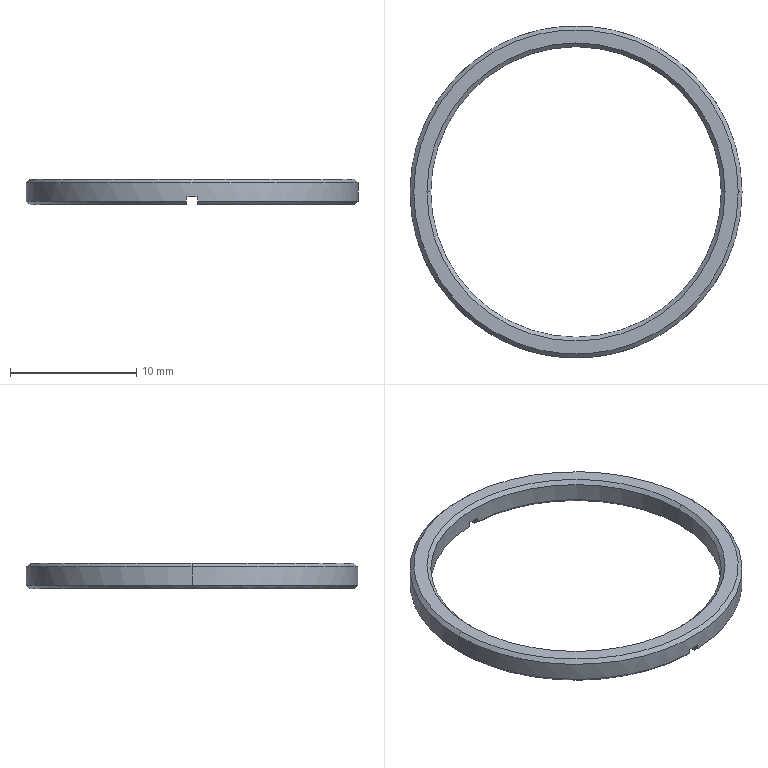Part | STEP file | 1 solid | 27 faces | box 26.29 x 26.29 x 2.05 mm | volume 245.399 mm3 | cone 10 | plane 9 | cylinder 8 | commonest cylinder face diameters 0.1 x4 23 x2 26.29 x2
STEP:
#1=CARTESIAN_POINT('',(12.845,0.,2.05));
#2=VERTEX_POINT('',#1);
#3=CARTESIAN_POINT('',(-12.845,0.,2.05));
#4=VERTEX_POINT('',#3);
#5=CARTESIAN_POINT('',(0.,0.,2.05));
#6=DIRECTION('',(0.,0.,1.));
#7=DIRECTION('',(1.,0.,0.));
#8=AXIS2_PLACEMENT_3D('',#5,#6,#7);
#9=CIRCLE('',#8,12.845);
#10=EDGE_CURVE('',#2,#4,#9,.T.);
#11=ORIENTED_EDGE('',*,*,#10,.F.);
#12=CARTESIAN_POINT('',(13.145,0.,1.75));
#13=VERTEX_POINT('',#12);
#14=CARTESIAN_POINT('',(12.845,0.,2.05));
#15=DIRECTION('',(0.7071,0.,-0.7071));
#16=VECTOR('',#15,1000.);
#17=LINE('',#14,#16);
#18=EDGE_CURVE('',#2,#13,#17,.T.);
#19=ORIENTED_EDGE('',*,*,#18,.T.);
#20=CARTESIAN_POINT('',(-13.145,0.,1.75));
#21=VERTEX_POINT('',#20);
#22=CARTESIAN_POINT('',(0.,0.,1.75));
#23=DIRECTION('',(0.,0.,-1.));
#24=DIRECTION('',(1.,0.,0.));
#25=AXIS2_PLACEMENT_3D('',#22,#23,#24);
#26=CIRCLE('',#25,13.145);
#27=EDGE_CURVE('',#21,#13,#26,.T.);
#28=ORIENTED_EDGE('',*,*,#27,.F.);
#29=CARTESIAN_POINT('',(-12.845,0.,2.05));
#30=DIRECTION('',(-0.7071,0.,-0.7071));
#31=VECTOR('',#30,1000.);
#32=LINE('',#29,#31);
#33=EDGE_CURVE('',#4,#21,#32,.T.);
#34=ORIENTED_EDGE('',*,*,#33,.F.);
#35=EDGE_LOOP('',(#11,#19,#28,#34));
#36=FACE_OUTER_BOUND('',#35,.T.);
#37=CARTESIAN_POINT('',(0.,0.,2.05));
#38=DIRECTION('',(0.,0.,-1.));
#39=DIRECTION('',(-1.,0.,0.));
#40=AXIS2_PLACEMENT_3D('',#37,#38,#39);
#41=CONICAL_SURFACE('',#40,12.845,0.7854);
#42=ADVANCED_FACE('',(#36),#41,.T.);
#43=CARTESIAN_POINT('',(-11.5,0.,1.75));
#44=VERTEX_POINT('',#43);
#45=CARTESIAN_POINT('',(11.5,0.,1.75));
#46=VERTEX_POINT('',#45);
#47=CARTESIAN_POINT('',(0.,0.,1.75));
#48=DIRECTION('',(0.,0.,1.));
#49=DIRECTION('',(1.,0.,0.));
#50=AXIS2_PLACEMENT_3D('',#47,#48,#49);
#51=CIRCLE('',#50,11.5);
#52=EDGE_CURVE('',#44,#46,#51,.T.);
#53=ORIENTED_EDGE('',*,*,#52,.F.);
#54=CARTESIAN_POINT('',(-11.8,0.,2.05));
#55=VERTEX_POINT('',#54);
#56=CARTESIAN_POINT('',(-11.5,0.,1.75));
#57=DIRECTION('',(-0.7071,0.,0.7071));
#58=VECTOR('',#57,1000.);
#59=LINE('',#56,#58);
#60=EDGE_CURVE('',#44,#55,#59,.T.);
#61=ORIENTED_EDGE('',*,*,#60,.T.);
#62=CARTESIAN_POINT('',(11.8,0.,2.05));
#63=VERTEX_POINT('',#62);
#64=CARTESIAN_POINT('',(0.,0.,2.05));
#65=DIRECTION('',(0.,0.,-1.));
#66=DIRECTION('',(1.,0.,0.));
#67=AXIS2_PLACEMENT_3D('',#64,#65,#66);
#68=CIRCLE('',#67,11.8);
#69=EDGE_CURVE('',#63,#55,#68,.T.);
#70=ORIENTED_EDGE('',*,*,#69,.F.);
#71=CARTESIAN_POINT('',(11.5,0.,1.75));
#72=DIRECTION('',(0.7071,0.,0.7071));
#73=VECTOR('',#72,1000.);
#74=LINE('',#71,#73);
#75=EDGE_CURVE('',#46,#63,#74,.T.);
#76=ORIENTED_EDGE('',*,*,#75,.F.);
#77=EDGE_LOOP('',(#53,#61,#70,#76));
#78=FACE_OUTER_BOUND('',#77,.T.);
#79=CARTESIAN_POINT('',(0.,0.,1.75));
#80=DIRECTION('',(0.,0.,1.));
#81=DIRECTION('',(1.,0.,0.));
#82=AXIS2_PLACEMENT_3D('',#79,#80,#81);
#83=CONICAL_SURFACE('',#82,11.5,0.7854);
#84=ADVANCED_FACE('',(#78),#83,.F.);
#85=CARTESIAN_POINT('',(-11.5,0.,0.3));
#86=VERTEX_POINT('',#85);
#87=CARTESIAN_POINT('',(-0.45,11.491,0.3));
#88=VERTEX_POINT('',#87);
#89=CARTESIAN_POINT('',(0.,0.,0.3));
#90=DIRECTION('',(0.,0.,-1.));
#91=DIRECTION('',(1.,0.,0.));
#92=AXIS2_PLACEMENT_3D('',#89,#90,#91);
#93=CIRCLE('',#92,11.5);
#94=EDGE_CURVE('',#86,#88,#93,.T.);
#95=ORIENTED_EDGE('',*,*,#94,.F.);
#96=CARTESIAN_POINT('',(-11.8,0.,0.));
#97=VERTEX_POINT('',#96);
#98=CARTESIAN_POINT('',(-11.8,0.,0.));
#99=DIRECTION('',(-0.7071,0.,-0.7071));
#100=VECTOR('',#99,1000.);
#101=LINE('',#98,#100);
#102=EDGE_CURVE('',#86,#97,#101,.T.);
#103=ORIENTED_EDGE('',*,*,#102,.T.);
#104=CARTESIAN_POINT('',(-0.45,11.791,0.));
#105=VERTEX_POINT('',#104);
#106=CARTESIAN_POINT('',(0.,0.,0.));
#107=DIRECTION('',(0.,0.,1.));
#108=DIRECTION('',(1.,0.,0.));
#109=AXIS2_PLACEMENT_3D('',#106,#107,#108);
#110=CIRCLE('',#109,11.8);
#111=EDGE_CURVE('',#105,#97,#110,.T.);
#112=ORIENTED_EDGE('',*,*,#111,.F.);
#113=CARTESIAN_POINT('',(-0.45,11.491,0.3));
#114=CARTESIAN_POINT('',(-0.45,11.591,0.2));
#115=CARTESIAN_POINT('',(-0.45,11.691,0.1));
#116=CARTESIAN_POINT('',(-0.45,11.791,0.));
#117=B_SPLINE_CURVE_WITH_KNOTS('',3,(#113,#114,#115,#116),.UNSPECIFIED.,.F.,.F.,(4,4),(0.05246,0.05288),.UNSPECIFIED.);
#118=EDGE_CURVE('',#88,#105,#117,.T.);
#119=ORIENTED_EDGE('',*,*,#118,.F.);
#120=EDGE_LOOP('',(#95,#103,#112,#119));
#121=FACE_OUTER_BOUND('',#120,.T.);
#122=CARTESIAN_POINT('',(0.,0.,0.));
#123=DIRECTION('',(0.,0.,-1.));
#124=DIRECTION('',(-1.,0.,0.));
#125=AXIS2_PLACEMENT_3D('',#122,#123,#124);
#126=CONICAL_SURFACE('',#125,11.8,0.7854);
#127=ADVANCED_FACE('',(#121),#126,.F.);
#128=ORIENTED_EDGE('',*,*,#52,.T.);
#129=CARTESIAN_POINT('',(11.5,0.,0.3));
#130=VERTEX_POINT('',#129);
#131=CARTESIAN_POINT('',(11.5,0.,2.05));
#132=DIRECTION('',(0.,0.,-1.));
#133=VECTOR('',#132,1000.);
#134=LINE('',#131,#133);
#135=EDGE_CURVE('',#46,#130,#134,.T.);
#136=ORIENTED_EDGE('',*,*,#135,.T.);
#137=CARTESIAN_POINT('',(0.45,-11.491,0.3));
#138=VERTEX_POINT('',#137);
#139=CARTESIAN_POINT('',(0.,0.,0.3));
#140=DIRECTION('',(0.,0.,-1.));
#141=DIRECTION('',(1.,0.,0.));
#142=AXIS2_PLACEMENT_3D('',#139,#140,#141);
#143=CIRCLE('',#142,11.5);
#144=EDGE_CURVE('',#130,#138,#143,.T.);
#145=ORIENTED_EDGE('',*,*,#144,.T.);
#146=CARTESIAN_POINT('',(0.45,-11.491,0.6));
#147=VERTEX_POINT('',#146);
#148=CARTESIAN_POINT('',(0.45,-11.491,2.05));
#149=DIRECTION('',(0.,0.,-1.));
#150=VECTOR('',#149,1000.);
#151=LINE('',#148,#150);
#152=EDGE_CURVE('',#147,#138,#151,.T.);
#153=ORIENTED_EDGE('',*,*,#152,.F.);
#154=CARTESIAN_POINT('',(0.4,-11.493,0.65));
#155=VERTEX_POINT('',#154);
#156=CARTESIAN_POINT('',(0.45,-11.491,0.6));
#157=CARTESIAN_POINT('',(0.45,-11.491,0.6056));
#158=CARTESIAN_POINT('',(0.449,-11.491,0.6113));
#159=CARTESIAN_POINT('',(0.4472,-11.491,0.6165));
#160=CARTESIAN_POINT('',(0.4453,-11.491,0.6218));
#161=CARTESIAN_POINT('',(0.4425,-11.491,0.6268));
#162=CARTESIAN_POINT('',(0.4391,-11.492,0.6312));
#163=CARTESIAN_POINT('',(0.4356,-11.492,0.6356));
#164=CARTESIAN_POINT('',(0.4313,-11.492,0.6394));
#165=CARTESIAN_POINT('',(0.4265,-11.492,0.6424));
#166=CARTESIAN_POINT('',(0.4218,-11.492,0.6453));
#167=CARTESIAN_POINT('',(0.4165,-11.492,0.6475));
#168=CARTESIAN_POINT('',(0.411,-11.493,0.6488));
#169=CARTESIAN_POINT('',(0.4074,-11.493,0.6496));
#170=CARTESIAN_POINT('',(0.4037,-11.493,0.65));
#171=CARTESIAN_POINT('',(0.4,-11.493,0.65));
#172=B_SPLINE_CURVE_WITH_KNOTS('',3,(#156,#157,#158,#159,#160,#161,#162,#163,#164,#165,#166,#167,#168,#169,#170,#171),.UNSPECIFIED.,.F.,.F.,(4,3,3,3,3,4),(0.,0.00001678,0.00003356,0.00005034,0.00006714,0.00007813),.UNSPECIFIED.);
#173=EDGE_CURVE('',#147,#155,#172,.T.);
#174=ORIENTED_EDGE('',*,*,#173,.T.);
#175=CARTESIAN_POINT('',(-0.4,-11.493,0.65));
#176=VERTEX_POINT('',#175);
#177=CARTESIAN_POINT('',(0.,0.,0.65));
#178=DIRECTION('',(0.,0.,-1.));
#179=DIRECTION('',(-1.,0.,0.));
#180=AXIS2_PLACEMENT_3D('',#177,#178,#179);
#181=CIRCLE('',#180,11.5);
#182=EDGE_CURVE('',#155,#176,#181,.T.);
#183=ORIENTED_EDGE('',*,*,#182,.T.);
#184=CARTESIAN_POINT('',(-0.45,-11.491,0.6));
#185=VERTEX_POINT('',#184);
#186=CARTESIAN_POINT('',(-0.4,-11.493,0.65));
#187=CARTESIAN_POINT('',(-0.4056,-11.493,0.65));
#188=CARTESIAN_POINT('',(-0.4113,-11.493,0.649));
#189=CARTESIAN_POINT('',(-0.4166,-11.492,0.6472));
#190=CARTESIAN_POINT('',(-0.4218,-11.492,0.6453));
#191=CARTESIAN_POINT('',(-0.4269,-11.492,0.6425));
#192=CARTESIAN_POINT('',(-0.4313,-11.492,0.639));
#193=CARTESIAN_POINT('',(-0.4356,-11.492,0.6355));
#194=CARTESIAN_POINT('',(-0.4394,-11.492,0.6312));
#195=CARTESIAN_POINT('',(-0.4424,-11.491,0.6265));
#196=CARTESIAN_POINT('',(-0.4454,-11.491,0.6217));
#197=CARTESIAN_POINT('',(-0.4476,-11.491,0.6164));
#198=CARTESIAN_POINT('',(-0.4488,-11.491,0.6109));
#199=CARTESIAN_POINT('',(-0.4496,-11.491,0.6074));
#200=CARTESIAN_POINT('',(-0.45,-11.491,0.6037));
#201=CARTESIAN_POINT('',(-0.45,-11.491,0.6));
#202=B_SPLINE_CURVE_WITH_KNOTS('',3,(#186,#187,#188,#189,#190,#191,#192,#193,#194,#195,#196,#197,#198,#199,#200,#201),.UNSPECIFIED.,.F.,.F.,(4,3,3,3,3,4),(0.,0.00001681,0.00003362,0.00005042,0.00006721,0.00007813),.UNSPECIFIED.);
#203=EDGE_CURVE('',#176,#185,#202,.T.);
#204=ORIENTED_EDGE('',*,*,#203,.T.);
#205=CARTESIAN_POINT('',(-0.45,-11.491,0.3));
#206=VERTEX_POINT('',#205);
#207=CARTESIAN_POINT('',(-0.45,-11.491,2.05));
#208=DIRECTION('',(0.,0.,1.));
#209=VECTOR('',#208,1000.);
#210=LINE('',#207,#209);
#211=EDGE_CURVE('',#206,#185,#210,.T.);
#212=ORIENTED_EDGE('',*,*,#211,.F.);
#213=CARTESIAN_POINT('',(0.,0.,0.3));
#214=DIRECTION('',(0.,0.,-1.));
#215=DIRECTION('',(1.,0.,0.));
#216=AXIS2_PLACEMENT_3D('',#213,#214,#215);
#217=CIRCLE('',#216,11.5);
#218=EDGE_CURVE('',#206,#86,#217,.T.);
#219=ORIENTED_EDGE('',*,*,#218,.T.);
#220=CARTESIAN_POINT('',(-11.5,0.,2.05));
#221=DIRECTION('',(0.,0.,-1.));
#222=VECTOR('',#221,1000.);
#223=LINE('',#220,#222);
#224=EDGE_CURVE('',#44,#86,#223,.T.);
#225=ORIENTED_EDGE('',*,*,#224,.F.);
#226=EDGE_LOOP('',(#128,#136,#145,#153,#174,#183,#204,#212,#219,#225));
#227=FACE_OUTER_BOUND('',#226,.T.);
#228=CARTESIAN_POINT('',(0.,0.,2.05));
#229=DIRECTION('',(0.,0.,-1.));
#230=DIRECTION('',(-1.,0.,0.));
#231=AXIS2_PLACEMENT_3D('',#228,#229,#230);
#232=CYLINDRICAL_SURFACE('',#231,11.5);
#233=ADVANCED_FACE('',(#227),#232,.F.);
#234=ORIENTED_EDGE('',*,*,#27,.T.);
#235=CARTESIAN_POINT('',(13.145,0.,0.3));
#236=VERTEX_POINT('',#235);
#237=CARTESIAN_POINT('',(13.145,0.,2.05));
#238=DIRECTION('',(0.,0.,-1.));
#239=VECTOR('',#238,1000.);
#240=LINE('',#237,#239);
#241=EDGE_CURVE('',#13,#236,#240,.T.);
#242=ORIENTED_EDGE('',*,*,#241,.T.);
#243=CARTESIAN_POINT('',(0.45,13.137,0.3));
#244=VERTEX_POINT('',#243);
#245=CARTESIAN_POINT('',(0.,0.,0.3));
#246=DIRECTION('',(0.,0.,1.));
#247=DIRECTION('',(1.,0.,0.));
#248=AXIS2_PLACEMENT_3D('',#245,#246,#247);
#249=CIRCLE('',#248,13.145);
#250=EDGE_CURVE('',#236,#244,#249,.T.);
#251=ORIENTED_EDGE('',*,*,#250,.T.);
#252=CARTESIAN_POINT('',(0.45,13.137,0.6));
#253=VERTEX_POINT('',#252);
#254=CARTESIAN_POINT('',(0.45,13.137,2.05));
#255=DIRECTION('',(0.,0.,1.));
#256=VECTOR('',#255,1000.);
#257=LINE('',#254,#256);
#258=EDGE_CURVE('',#244,#253,#257,.T.);
#259=ORIENTED_EDGE('',*,*,#258,.T.);
#260=CARTESIAN_POINT('',(0.4,13.139,0.65));
#261=VERTEX_POINT('',#260);
#262=CARTESIAN_POINT('',(0.45,13.137,0.6));
#263=CARTESIAN_POINT('',(0.45,13.137,0.6056));
#264=CARTESIAN_POINT('',(0.449,13.137,0.6113));
#265=CARTESIAN_POINT('',(0.4472,13.137,0.6165));
#266=CARTESIAN_POINT('',(0.4453,13.137,0.6218));
#267=CARTESIAN_POINT('',(0.4425,13.138,0.6269));
#268=CARTESIAN_POINT('',(0.4391,13.138,0.6312));
#269=CARTESIAN_POINT('',(0.4356,13.138,0.6356));
#270=CARTESIAN_POINT('',(0.4313,13.138,0.6394));
#271=CARTESIAN_POINT('',(0.4265,13.138,0.6424));
#272=CARTESIAN_POINT('',(0.4218,13.138,0.6454));
#273=CARTESIAN_POINT('',(0.4165,13.138,0.6475));
#274=CARTESIAN_POINT('',(0.411,13.139,0.6488));
#275=CARTESIAN_POINT('',(0.4074,13.139,0.6496));
#276=CARTESIAN_POINT('',(0.4037,13.139,0.65));
#277=CARTESIAN_POINT('',(0.4,13.139,0.65));
#278=B_SPLINE_CURVE_WITH_KNOTS('',3,(#262,#263,#264,#265,#266,#267,#268,#269,#270,#271,#272,#273,#274,#275,#276,#277),.UNSPECIFIED.,.F.,.F.,(4,3,3,3,3,4),(0.,0.00001678,0.00003356,0.00005035,0.00006714,0.00007813),.UNSPECIFIED.);
#279=EDGE_CURVE('',#253,#261,#278,.T.);
#280=ORIENTED_EDGE('',*,*,#279,.T.);
#281=CARTESIAN_POINT('',(-0.4,13.139,0.65));
#282=VERTEX_POINT('',#281);
#283=CARTESIAN_POINT('',(0.,0.,0.65));
#284=DIRECTION('',(0.,0.,-1.));
#285=DIRECTION('',(-1.,0.,0.));
#286=AXIS2_PLACEMENT_3D('',#283,#284,#285);
#287=CIRCLE('',#286,13.145);
#288=EDGE_CURVE('',#282,#261,#287,.T.);
#289=ORIENTED_EDGE('',*,*,#288,.F.);
#290=CARTESIAN_POINT('',(-0.45,13.137,0.6));
#291=VERTEX_POINT('',#290);
#292=CARTESIAN_POINT('',(-0.4,13.139,0.65));
#293=CARTESIAN_POINT('',(-0.4056,13.139,0.65));
#294=CARTESIAN_POINT('',(-0.4113,13.139,0.649));
#295=CARTESIAN_POINT('',(-0.4166,13.138,0.6472));
#296=CARTESIAN_POINT('',(-0.4218,13.138,0.6453));
#297=CARTESIAN_POINT('',(-0.4269,13.138,0.6425));
#298=CARTESIAN_POINT('',(-0.4312,13.138,0.639));
#299=CARTESIAN_POINT('',(-0.4356,13.138,0.6355));
#300=CARTESIAN_POINT('',(-0.4394,13.138,0.6312));
#301=CARTESIAN_POINT('',(-0.4424,13.138,0.6265));
#302=CARTESIAN_POINT('',(-0.4454,13.137,0.6217));
#303=CARTESIAN_POINT('',(-0.4476,13.137,0.6164));
#304=CARTESIAN_POINT('',(-0.4488,13.137,0.611));
#305=CARTESIAN_POINT('',(-0.4496,13.137,0.6074));
#306=CARTESIAN_POINT('',(-0.45,13.137,0.6037));
#307=CARTESIAN_POINT('',(-0.45,13.137,0.6));
#308=B_SPLINE_CURVE_WITH_KNOTS('',3,(#292,#293,#294,#295,#296,#297,#298,#299,#300,#301,#302,#303,#304,#305,#306,#307),.UNSPECIFIED.,.F.,.F.,(4,3,3,3,3,4),(0.,0.0000168,0.00003361,0.00005041,0.0000672,0.00007813),.UNSPECIFIED.);
#309=EDGE_CURVE('',#282,#291,#308,.T.);
#310=ORIENTED_EDGE('',*,*,#309,.T.);
#311=CARTESIAN_POINT('',(-0.45,13.137,0.3));
#312=VERTEX_POINT('',#311);
#313=CARTESIAN_POINT('',(-0.45,13.137,2.05));
#314=DIRECTION('',(0.,0.,-1.));
#315=VECTOR('',#314,1000.);
#316=LINE('',#313,#315);
#317=EDGE_CURVE('',#291,#312,#316,.T.);
#318=ORIENTED_EDGE('',*,*,#317,.T.);
#319=CARTESIAN_POINT('',(-13.145,0.,0.3));
#320=VERTEX_POINT('',#319);
#321=CARTESIAN_POINT('',(0.,0.,0.3));
#322=DIRECTION('',(0.,0.,1.));
#323=DIRECTION('',(1.,0.,0.));
#324=AXIS2_PLACEMENT_3D('',#321,#322,#323);
#325=CIRCLE('',#324,13.145);
#326=EDGE_CURVE('',#312,#320,#325,.T.);
#327=ORIENTED_EDGE('',*,*,#326,.T.);
#328=CARTESIAN_POINT('',(-13.145,0.,2.05));
#329=DIRECTION('',(0.,0.,-1.));
#330=VECTOR('',#329,1000.);
#331=LINE('',#328,#330);
#332=EDGE_CURVE('',#21,#320,#331,.T.);
#333=ORIENTED_EDGE('',*,*,#332,.F.);
#334=EDGE_LOOP('',(#234,#242,#251,#259,#280,#289,#310,#318,#327,#333));
#335=FACE_OUTER_BOUND('',#334,.T.);
#336=CARTESIAN_POINT('',(0.,0.,2.05));
#337=DIRECTION('',(0.,0.,-1.));
#338=DIRECTION('',(-1.,0.,0.));
#339=AXIS2_PLACEMENT_3D('',#336,#337,#338);
#340=CYLINDRICAL_SURFACE('',#339,13.145);
#341=ADVANCED_FACE('',(#335),#340,.T.);
#342=CARTESIAN_POINT('',(12.845,0.,0.));
#343=VERTEX_POINT('',#342);
#344=CARTESIAN_POINT('',(0.45,-12.837,0.));
#345=VERTEX_POINT('',#344);
#346=CARTESIAN_POINT('',(0.,0.,0.));
#347=DIRECTION('',(0.,0.,-1.));
#348=DIRECTION('',(1.,0.,0.));
#349=AXIS2_PLACEMENT_3D('',#346,#347,#348);
#350=CIRCLE('',#349,12.845);
#351=EDGE_CURVE('',#343,#345,#350,.T.);
#352=ORIENTED_EDGE('',*,*,#351,.F.);
#353=CARTESIAN_POINT('',(13.145,0.,0.3));
#354=DIRECTION('',(0.7071,0.,0.7071));
#355=VECTOR('',#354,1000.);
#356=LINE('',#353,#355);
#357=EDGE_CURVE('',#343,#236,#356,.T.);
#358=ORIENTED_EDGE('',*,*,#357,.T.);
#359=CARTESIAN_POINT('',(0.45,-13.137,0.3));
#360=VERTEX_POINT('',#359);
#361=CARTESIAN_POINT('',(0.,0.,0.3));
#362=DIRECTION('',(0.,0.,1.));
#363=DIRECTION('',(1.,0.,0.));
#364=AXIS2_PLACEMENT_3D('',#361,#362,#363);
#365=CIRCLE('',#364,13.145);
#366=EDGE_CURVE('',#360,#236,#365,.T.);
#367=ORIENTED_EDGE('',*,*,#366,.F.);
#368=CARTESIAN_POINT('',(0.45,-12.837,0.));
#369=CARTESIAN_POINT('',(0.45,-12.937,0.1));
#370=CARTESIAN_POINT('',(0.45,-13.037,0.2));
#371=CARTESIAN_POINT('',(0.45,-13.137,0.3));
#372=B_SPLINE_CURVE_WITH_KNOTS('',3,(#368,#369,#370,#371),.UNSPECIFIED.,.F.,.F.,(4,4),(0.05853,0.05895),.UNSPECIFIED.);
#373=EDGE_CURVE('',#345,#360,#372,.T.);
#374=ORIENTED_EDGE('',*,*,#373,.F.);
#375=EDGE_LOOP('',(#352,#358,#367,#374));
#376=FACE_OUTER_BOUND('',#375,.T.);
#377=CARTESIAN_POINT('',(0.,0.,0.3));
#378=DIRECTION('',(0.,0.,1.));
#379=DIRECTION('',(1.,0.,0.));
#380=AXIS2_PLACEMENT_3D('',#377,#378,#379);
#381=CONICAL_SURFACE('',#380,13.145,0.7854);
#382=ADVANCED_FACE('',(#376),#381,.T.);
#383=CARTESIAN_POINT('',(0.45,12.837,0.));
#384=VERTEX_POINT('',#383);
#385=CARTESIAN_POINT('',(0.,0.,0.));
#386=DIRECTION('',(0.,0.,-1.));
#387=DIRECTION('',(1.,0.,0.));
#388=AXIS2_PLACEMENT_3D('',#385,#386,#387);
#389=CIRCLE('',#388,12.845);
#390=EDGE_CURVE('',#384,#343,#389,.T.);
#391=ORIENTED_EDGE('',*,*,#390,.T.);
#392=ORIENTED_EDGE('',*,*,#351,.T.);
#393=CARTESIAN_POINT('',(0.45,-11.791,0.));
#394=VERTEX_POINT('',#393);
#395=CARTESIAN_POINT('',(0.45,14.718,0.));
#396=DIRECTION('',(0.,-1.,0.));
#397=VECTOR('',#396,1000.);
#398=LINE('',#395,#397);
#399=EDGE_CURVE('',#394,#345,#398,.T.);
#400=ORIENTED_EDGE('',*,*,#399,.F.);
#401=CARTESIAN_POINT('',(0.45,11.791,0.));
#402=VERTEX_POINT('',#401);
#403=CARTESIAN_POINT('',(0.,0.,0.));
#404=DIRECTION('',(0.,0.,1.));
#405=DIRECTION('',(1.,0.,0.));
#406=AXIS2_PLACEMENT_3D('',#403,#404,#405);
#407=CIRCLE('',#406,11.8);
#408=EDGE_CURVE('',#394,#402,#407,.T.);
#409=ORIENTED_EDGE('',*,*,#408,.T.);
#410=CARTESIAN_POINT('',(0.45,14.718,0.));
#411=DIRECTION('',(0.,-1.,0.));
#412=VECTOR('',#411,1000.);
#413=LINE('',#410,#412);
#414=EDGE_CURVE('',#384,#402,#413,.T.);
#415=ORIENTED_EDGE('',*,*,#414,.F.);
#416=EDGE_LOOP('',(#391,#392,#400,#409,#415));
#417=FACE_OUTER_BOUND('',#416,.T.);
#418=CARTESIAN_POINT('',(0.,0.,0.));
#419=DIRECTION('',(0.,0.,1.));
#420=DIRECTION('',(1.,0.,0.));
#421=AXIS2_PLACEMENT_3D('',#418,#419,#420);
#422=PLANE('',#421);
#423=ADVANCED_FACE('',(#417),#422,.F.);
#424=CARTESIAN_POINT('',(0.45,11.491,0.3));
#425=VERTEX_POINT('',#424);
#426=CARTESIAN_POINT('',(0.45,11.791,0.));
#427=CARTESIAN_POINT('',(0.45,11.691,0.1));
#428=CARTESIAN_POINT('',(0.45,11.591,0.2));
#429=CARTESIAN_POINT('',(0.45,11.491,0.3));
#430=B_SPLINE_CURVE_WITH_KNOTS('',3,(#426,#427,#428,#429),.UNSPECIFIED.,.F.,.F.,(4,4),(0.02003,0.02045),.UNSPECIFIED.);
#431=EDGE_CURVE('',#402,#425,#430,.T.);
#432=ORIENTED_EDGE('',*,*,#431,.F.);
#433=ORIENTED_EDGE('',*,*,#408,.F.);
#434=CARTESIAN_POINT('',(0.45,-11.491,0.3));
#435=CARTESIAN_POINT('',(0.45,-11.591,0.2));
#436=CARTESIAN_POINT('',(0.45,-11.691,0.1));
#437=CARTESIAN_POINT('',(0.45,-11.791,0.));
#438=B_SPLINE_CURVE_WITH_KNOTS('',3,(#434,#435,#436,#437),.UNSPECIFIED.,.F.,.F.,(4,4),(0.05246,0.05288),.UNSPECIFIED.);
#439=EDGE_CURVE('',#138,#394,#438,.T.);
#440=ORIENTED_EDGE('',*,*,#439,.F.);
#441=ORIENTED_EDGE('',*,*,#144,.F.);
#442=CARTESIAN_POINT('',(0.,0.,0.3));
#443=DIRECTION('',(0.,0.,-1.));
#444=DIRECTION('',(1.,0.,0.));
#445=AXIS2_PLACEMENT_3D('',#442,#443,#444);
#446=CIRCLE('',#445,11.5);
#447=EDGE_CURVE('',#425,#130,#446,.T.);
#448=ORIENTED_EDGE('',*,*,#447,.F.);
#449=EDGE_LOOP('',(#432,#433,#440,#441,#448));
#450=FACE_OUTER_BOUND('',#449,.T.);
#451=CARTESIAN_POINT('',(0.,0.,0.));
#452=DIRECTION('',(0.,0.,-1.));
#453=DIRECTION('',(-1.,0.,0.));
#454=AXIS2_PLACEMENT_3D('',#451,#452,#453);
#455=CONICAL_SURFACE('',#454,11.8,0.7854);
#456=ADVANCED_FACE('',(#450),#455,.F.);
#457=ORIENTED_EDGE('',*,*,#357,.F.);
#458=ORIENTED_EDGE('',*,*,#390,.F.);
#459=CARTESIAN_POINT('',(0.45,13.137,0.3));
#460=CARTESIAN_POINT('',(0.45,13.037,0.2));
#461=CARTESIAN_POINT('',(0.45,12.937,0.1));
#462=CARTESIAN_POINT('',(0.45,12.837,0.));
#463=B_SPLINE_CURVE_WITH_KNOTS('',3,(#459,#460,#461,#462),.UNSPECIFIED.,.F.,.F.,(4,4),(0.02231,0.02274),.UNSPECIFIED.);
#464=EDGE_CURVE('',#244,#384,#463,.T.);
#465=ORIENTED_EDGE('',*,*,#464,.F.);
#466=ORIENTED_EDGE('',*,*,#250,.F.);
#467=EDGE_LOOP('',(#457,#458,#465,#466));
#468=FACE_OUTER_BOUND('',#467,.T.);
#469=CARTESIAN_POINT('',(0.,0.,0.3));
#470=DIRECTION('',(0.,0.,1.));
#471=DIRECTION('',(1.,0.,0.));
#472=AXIS2_PLACEMENT_3D('',#469,#470,#471);
#473=CONICAL_SURFACE('',#472,13.145,0.7854);
#474=ADVANCED_FACE('',(#468),#473,.T.);
#475=ORIENTED_EDGE('',*,*,#69,.T.);
#476=CARTESIAN_POINT('',(0.,0.,2.05));
#477=DIRECTION('',(0.,0.,-1.));
#478=DIRECTION('',(1.,0.,0.));
#479=AXIS2_PLACEMENT_3D('',#476,#477,#478);
#480=CIRCLE('',#479,11.8);
#481=EDGE_CURVE('',#55,#63,#480,.T.);
#482=ORIENTED_EDGE('',*,*,#481,.T.);
#483=EDGE_LOOP('',(#475,#482));
#484=FACE_BOUND('',#483,.T.);
#485=CARTESIAN_POINT('',(0.,0.,2.05));
#486=DIRECTION('',(0.,0.,1.));
#487=DIRECTION('',(1.,0.,0.));
#488=AXIS2_PLACEMENT_3D('',#485,#486,#487);
#489=CIRCLE('',#488,12.845);
#490=EDGE_CURVE('',#4,#2,#489,.T.);
#491=ORIENTED_EDGE('',*,*,#490,.T.);
#492=ORIENTED_EDGE('',*,*,#10,.T.);
#493=EDGE_LOOP('',(#491,#492));
#494=FACE_OUTER_BOUND('',#493,.T.);
#495=CARTESIAN_POINT('',(0.,0.,2.05));
#496=DIRECTION('',(0.,0.,1.));
#497=DIRECTION('',(1.,0.,0.));
#498=AXIS2_PLACEMENT_3D('',#495,#496,#497);
#499=PLANE('',#498);
#500=ADVANCED_FACE('',(#484,#494),#499,.T.);
#501=CARTESIAN_POINT('',(-0.45,-12.837,0.));
#502=VERTEX_POINT('',#501);
#503=CARTESIAN_POINT('',(-0.45,12.837,0.));
#504=VERTEX_POINT('',#503);
#505=CARTESIAN_POINT('',(0.,0.,0.));
#506=DIRECTION('',(0.,0.,-1.));
#507=DIRECTION('',(1.,0.,0.));
#508=AXIS2_PLACEMENT_3D('',#505,#506,#507);
#509=CIRCLE('',#508,12.845);
#510=EDGE_CURVE('',#502,#504,#509,.T.);
#511=ORIENTED_EDGE('',*,*,#510,.T.);
#512=CARTESIAN_POINT('',(-0.45,14.718,0.));
#513=DIRECTION('',(0.,1.,0.));
#514=VECTOR('',#513,1000.);
#515=LINE('',#512,#514);
#516=EDGE_CURVE('',#105,#504,#515,.T.);
#517=ORIENTED_EDGE('',*,*,#516,.F.);
#518=ORIENTED_EDGE('',*,*,#111,.T.);
#519=CARTESIAN_POINT('',(-0.45,-11.791,0.));
#520=VERTEX_POINT('',#519);
#521=CARTESIAN_POINT('',(0.,0.,0.));
#522=DIRECTION('',(0.,0.,1.));
#523=DIRECTION('',(1.,0.,0.));
#524=AXIS2_PLACEMENT_3D('',#521,#522,#523);
#525=CIRCLE('',#524,11.8);
#526=EDGE_CURVE('',#97,#520,#525,.T.);
#527=ORIENTED_EDGE('',*,*,#526,.T.);
#528=CARTESIAN_POINT('',(-0.45,14.718,0.));
#529=DIRECTION('',(0.,1.,0.));
#530=VECTOR('',#529,1000.);
#531=LINE('',#528,#530);
#532=EDGE_CURVE('',#502,#520,#531,.T.);
#533=ORIENTED_EDGE('',*,*,#532,.F.);
#534=EDGE_LOOP('',(#511,#517,#518,#527,#533));
#535=FACE_OUTER_BOUND('',#534,.T.);
#536=CARTESIAN_POINT('',(0.,0.,0.));
#537=DIRECTION('',(0.,0.,1.));
#538=DIRECTION('',(1.,0.,0.));
#539=AXIS2_PLACEMENT_3D('',#536,#537,#538);
#540=PLANE('',#539);
#541=ADVANCED_FACE('',(#535),#540,.F.);
#542=ORIENTED_EDGE('',*,*,#241,.F.);
#543=CARTESIAN_POINT('',(0.,0.,1.75));
#544=DIRECTION('',(0.,0.,-1.));
#545=DIRECTION('',(1.,0.,0.));
#546=AXIS2_PLACEMENT_3D('',#543,#544,#545);
#547=CIRCLE('',#546,13.145);
#548=EDGE_CURVE('',#13,#21,#547,.T.);
#549=ORIENTED_EDGE('',*,*,#548,.T.);
#550=ORIENTED_EDGE('',*,*,#332,.T.);
#551=CARTESIAN_POINT('',(-0.45,-13.137,0.3));
#552=VERTEX_POINT('',#551);
#553=CARTESIAN_POINT('',(0.,0.,0.3));
#554=DIRECTION('',(0.,0.,1.));
#555=DIRECTION('',(1.,0.,0.));
#556=AXIS2_PLACEMENT_3D('',#553,#554,#555);
#557=CIRCLE('',#556,13.145);
#558=EDGE_CURVE('',#320,#552,#557,.T.);
#559=ORIENTED_EDGE('',*,*,#558,.T.);
#560=CARTESIAN_POINT('',(-0.45,-13.137,0.6));
#561=VERTEX_POINT('',#560);
#562=CARTESIAN_POINT('',(-0.45,-13.137,2.05));
#563=DIRECTION('',(0.,0.,1.));
#564=VECTOR('',#563,1000.);
#565=LINE('',#562,#564);
#566=EDGE_CURVE('',#552,#561,#565,.T.);
#567=ORIENTED_EDGE('',*,*,#566,.T.);
#568=CARTESIAN_POINT('',(-0.4,-13.139,0.65));
#569=VERTEX_POINT('',#568);
#570=CARTESIAN_POINT('',(-0.45,-13.137,0.6));
#571=CARTESIAN_POINT('',(-0.45,-13.137,0.6056));
#572=CARTESIAN_POINT('',(-0.449,-13.137,0.6113));
#573=CARTESIAN_POINT('',(-0.4472,-13.137,0.6165));
#574=CARTESIAN_POINT('',(-0.4453,-13.137,0.6218));
#575=CARTESIAN_POINT('',(-0.4425,-13.138,0.6269));
#576=CARTESIAN_POINT('',(-0.4391,-13.138,0.6312));
#577=CARTESIAN_POINT('',(-0.4356,-13.138,0.6356));
#578=CARTESIAN_POINT('',(-0.4313,-13.138,0.6394));
#579=CARTESIAN_POINT('',(-0.4265,-13.138,0.6424));
#580=CARTESIAN_POINT('',(-0.4218,-13.138,0.6454));
#581=CARTESIAN_POINT('',(-0.4165,-13.138,0.6475));
#582=CARTESIAN_POINT('',(-0.411,-13.139,0.6488));
#583=CARTESIAN_POINT('',(-0.4074,-13.139,0.6496));
#584=CARTESIAN_POINT('',(-0.4037,-13.139,0.65));
#585=CARTESIAN_POINT('',(-0.4,-13.139,0.65));
#586=B_SPLINE_CURVE_WITH_KNOTS('',3,(#570,#571,#572,#573,#574,#575,#576,#577,#578,#579,#580,#581,#582,#583,#584,#585),.UNSPECIFIED.,.F.,.F.,(4,3,3,3,3,4),(0.,0.00001678,0.00003356,0.00005035,0.00006714,0.00007813),.UNSPECIFIED.);
#587=EDGE_CURVE('',#561,#569,#586,.T.);
#588=ORIENTED_EDGE('',*,*,#587,.T.);
#589=CARTESIAN_POINT('',(0.4,-13.139,0.65));
#590=VERTEX_POINT('',#589);
#591=CARTESIAN_POINT('',(0.,0.,0.65));
#592=DIRECTION('',(0.,0.,-1.));
#593=DIRECTION('',(-1.,0.,0.));
#594=AXIS2_PLACEMENT_3D('',#591,#592,#593);
#595=CIRCLE('',#594,13.145);
#596=EDGE_CURVE('',#590,#569,#595,.T.);
#597=ORIENTED_EDGE('',*,*,#596,.F.);
#598=CARTESIAN_POINT('',(0.45,-13.137,0.6));
#599=VERTEX_POINT('',#598);
#600=CARTESIAN_POINT('',(0.4,-13.139,0.65));
#601=CARTESIAN_POINT('',(0.4056,-13.139,0.65));
#602=CARTESIAN_POINT('',(0.4113,-13.139,0.649));
#603=CARTESIAN_POINT('',(0.4166,-13.138,0.6472));
#604=CARTESIAN_POINT('',(0.4218,-13.138,0.6453));
#605=CARTESIAN_POINT('',(0.4269,-13.138,0.6425));
#606=CARTESIAN_POINT('',(0.4312,-13.138,0.639));
#607=CARTESIAN_POINT('',(0.4356,-13.138,0.6355));
#608=CARTESIAN_POINT('',(0.4394,-13.138,0.6312));
#609=CARTESIAN_POINT('',(0.4424,-13.138,0.6265));
#610=CARTESIAN_POINT('',(0.4454,-13.137,0.6217));
#611=CARTESIAN_POINT('',(0.4476,-13.137,0.6164));
#612=CARTESIAN_POINT('',(0.4488,-13.137,0.611));
#613=CARTESIAN_POINT('',(0.4496,-13.137,0.6074));
#614=CARTESIAN_POINT('',(0.45,-13.137,0.6037));
#615=CARTESIAN_POINT('',(0.45,-13.137,0.6));
#616=B_SPLINE_CURVE_WITH_KNOTS('',3,(#600,#601,#602,#603,#604,#605,#606,#607,#608,#609,#610,#611,#612,#613,#614,#615),.UNSPECIFIED.,.F.,.F.,(4,3,3,3,3,4),(0.,0.0000168,0.00003361,0.00005041,0.0000672,0.00007813),.UNSPECIFIED.);
#617=EDGE_CURVE('',#590,#599,#616,.T.);
#618=ORIENTED_EDGE('',*,*,#617,.T.);
#619=CARTESIAN_POINT('',(0.45,-13.137,2.05));
#620=DIRECTION('',(0.,0.,-1.));
#621=VECTOR('',#620,1000.);
#622=LINE('',#619,#621);
#623=EDGE_CURVE('',#599,#360,#622,.T.);
#624=ORIENTED_EDGE('',*,*,#623,.T.);
#625=ORIENTED_EDGE('',*,*,#366,.T.);
#626=EDGE_LOOP('',(#542,#549,#550,#559,#567,#588,#597,#618,#624,#625));
#627=FACE_OUTER_BOUND('',#626,.T.);
#628=CARTESIAN_POINT('',(0.,0.,2.05));
#629=DIRECTION('',(0.,0.,-1.));
#630=DIRECTION('',(-1.,0.,0.));
#631=AXIS2_PLACEMENT_3D('',#628,#629,#630);
#632=CYLINDRICAL_SURFACE('',#631,13.145);
#633=ADVANCED_FACE('',(#627),#632,.T.);
#634=ORIENTED_EDGE('',*,*,#135,.F.);
#635=CARTESIAN_POINT('',(0.,0.,1.75));
#636=DIRECTION('',(0.,0.,1.));
#637=DIRECTION('',(1.,0.,0.));
#638=AXIS2_PLACEMENT_3D('',#635,#636,#637);
#639=CIRCLE('',#638,11.5);
#640=EDGE_CURVE('',#46,#44,#639,.T.);
#641=ORIENTED_EDGE('',*,*,#640,.T.);
#642=ORIENTED_EDGE('',*,*,#224,.T.);
#643=ORIENTED_EDGE('',*,*,#94,.T.);
#644=CARTESIAN_POINT('',(-0.45,11.491,0.6));
#645=VERTEX_POINT('',#644);
#646=CARTESIAN_POINT('',(-0.45,11.491,2.05));
#647=DIRECTION('',(0.,0.,-1.));
#648=VECTOR('',#647,1000.);
#649=LINE('',#646,#648);
#650=EDGE_CURVE('',#645,#88,#649,.T.);
#651=ORIENTED_EDGE('',*,*,#650,.F.);
#652=CARTESIAN_POINT('',(-0.4,11.493,0.65));
#653=VERTEX_POINT('',#652);
#654=CARTESIAN_POINT('',(-0.45,11.491,0.6));
#655=CARTESIAN_POINT('',(-0.45,11.491,0.6056));
#656=CARTESIAN_POINT('',(-0.449,11.491,0.6113));
#657=CARTESIAN_POINT('',(-0.4472,11.491,0.6165));
#658=CARTESIAN_POINT('',(-0.4453,11.491,0.6218));
#659=CARTESIAN_POINT('',(-0.4425,11.491,0.6268));
#660=CARTESIAN_POINT('',(-0.4391,11.492,0.6312));
#661=CARTESIAN_POINT('',(-0.4356,11.492,0.6356));
#662=CARTESIAN_POINT('',(-0.4313,11.492,0.6394));
#663=CARTESIAN_POINT('',(-0.4265,11.492,0.6424));
#664=CARTESIAN_POINT('',(-0.4218,11.492,0.6453));
#665=CARTESIAN_POINT('',(-0.4165,11.492,0.6475));
#666=CARTESIAN_POINT('',(-0.411,11.493,0.6488));
#667=CARTESIAN_POINT('',(-0.4074,11.493,0.6496));
#668=CARTESIAN_POINT('',(-0.4037,11.493,0.65));
#669=CARTESIAN_POINT('',(-0.4,11.493,0.65));
#670=B_SPLINE_CURVE_WITH_KNOTS('',3,(#654,#655,#656,#657,#658,#659,#660,#661,#662,#663,#664,#665,#666,#667,#668,#669),.UNSPECIFIED.,.F.,.F.,(4,3,3,3,3,4),(0.,0.00001678,0.00003356,0.00005034,0.00006714,0.00007813),.UNSPECIFIED.);
#671=EDGE_CURVE('',#645,#653,#670,.T.);
#672=ORIENTED_EDGE('',*,*,#671,.T.);
#673=CARTESIAN_POINT('',(0.4,11.493,0.65));
#674=VERTEX_POINT('',#673);
#675=CARTESIAN_POINT('',(0.,0.,0.65));
#676=DIRECTION('',(0.,0.,-1.));
#677=DIRECTION('',(-1.,0.,0.));
#678=AXIS2_PLACEMENT_3D('',#675,#676,#677);
#679=CIRCLE('',#678,11.5);
#680=EDGE_CURVE('',#653,#674,#679,.T.);
#681=ORIENTED_EDGE('',*,*,#680,.T.);
#682=CARTESIAN_POINT('',(0.45,11.491,0.6));
#683=VERTEX_POINT('',#682);
#684=CARTESIAN_POINT('',(0.4,11.493,0.65));
#685=CARTESIAN_POINT('',(0.4056,11.493,0.65));
#686=CARTESIAN_POINT('',(0.4113,11.493,0.649));
#687=CARTESIAN_POINT('',(0.4166,11.492,0.6472));
#688=CARTESIAN_POINT('',(0.4218,11.492,0.6453));
#689=CARTESIAN_POINT('',(0.4269,11.492,0.6425));
#690=CARTESIAN_POINT('',(0.4313,11.492,0.639));
#691=CARTESIAN_POINT('',(0.4356,11.492,0.6355));
#692=CARTESIAN_POINT('',(0.4394,11.492,0.6312));
#693=CARTESIAN_POINT('',(0.4424,11.491,0.6265));
#694=CARTESIAN_POINT('',(0.4454,11.491,0.6217));
#695=CARTESIAN_POINT('',(0.4476,11.491,0.6164));
#696=CARTESIAN_POINT('',(0.4488,11.491,0.6109));
#697=CARTESIAN_POINT('',(0.4496,11.491,0.6074));
#698=CARTESIAN_POINT('',(0.45,11.491,0.6037));
#699=CARTESIAN_POINT('',(0.45,11.491,0.6));
#700=B_SPLINE_CURVE_WITH_KNOTS('',3,(#684,#685,#686,#687,#688,#689,#690,#691,#692,#693,#694,#695,#696,#697,#698,#699),.UNSPECIFIED.,.F.,.F.,(4,3,3,3,3,4),(0.,0.00001681,0.00003362,0.00005042,0.00006721,0.00007813),.UNSPECIFIED.);
#701=EDGE_CURVE('',#674,#683,#700,.T.);
#702=ORIENTED_EDGE('',*,*,#701,.T.);
#703=CARTESIAN_POINT('',(0.45,11.491,2.05));
#704=DIRECTION('',(0.,0.,1.));
#705=VECTOR('',#704,1000.);
#706=LINE('',#703,#705);
#707=EDGE_CURVE('',#425,#683,#706,.T.);
#708=ORIENTED_EDGE('',*,*,#707,.F.);
#709=ORIENTED_EDGE('',*,*,#447,.T.);
#710=EDGE_LOOP('',(#634,#641,#642,#643,#651,#672,#681,#702,#708,#709));
#711=FACE_OUTER_BOUND('',#710,.T.);
#712=CARTESIAN_POINT('',(0.,0.,2.05));
#713=DIRECTION('',(0.,0.,-1.));
#714=DIRECTION('',(-1.,0.,0.));
#715=AXIS2_PLACEMENT_3D('',#712,#713,#714);
#716=CYLINDRICAL_SURFACE('',#715,11.5);
#717=ADVANCED_FACE('',(#711),#716,.F.);
#718=ORIENTED_EDGE('',*,*,#102,.F.);
#719=ORIENTED_EDGE('',*,*,#218,.F.);
#720=CARTESIAN_POINT('',(-0.45,-11.791,0.));
#721=CARTESIAN_POINT('',(-0.45,-11.691,0.1));
#722=CARTESIAN_POINT('',(-0.45,-11.591,0.2));
#723=CARTESIAN_POINT('',(-0.45,-11.491,0.3));
#724=B_SPLINE_CURVE_WITH_KNOTS('',3,(#720,#721,#722,#723),.UNSPECIFIED.,.F.,.F.,(4,4),(0.02003,0.02045),.UNSPECIFIED.);
#725=EDGE_CURVE('',#520,#206,#724,.T.);
#726=ORIENTED_EDGE('',*,*,#725,.F.);
#727=ORIENTED_EDGE('',*,*,#526,.F.);
#728=EDGE_LOOP('',(#718,#719,#726,#727));
#729=FACE_OUTER_BOUND('',#728,.T.);
#730=CARTESIAN_POINT('',(0.,0.,0.));
#731=DIRECTION('',(0.,0.,-1.));
#732=DIRECTION('',(-1.,0.,0.));
#733=AXIS2_PLACEMENT_3D('',#730,#731,#732);
#734=CONICAL_SURFACE('',#733,11.8,0.7854);
#735=ADVANCED_FACE('',(#729),#734,.F.);
#736=ORIENTED_EDGE('',*,*,#60,.F.);
#737=ORIENTED_EDGE('',*,*,#640,.F.);
#738=ORIENTED_EDGE('',*,*,#75,.T.);
#739=ORIENTED_EDGE('',*,*,#481,.F.);
#740=EDGE_LOOP('',(#736,#737,#738,#739));
#741=FACE_OUTER_BOUND('',#740,.T.);
#742=CARTESIAN_POINT('',(0.,0.,1.75));
#743=DIRECTION('',(0.,0.,1.));
#744=DIRECTION('',(1.,0.,0.));
#745=AXIS2_PLACEMENT_3D('',#742,#743,#744);
#746=CONICAL_SURFACE('',#745,11.5,0.7854);
#747=ADVANCED_FACE('',(#741),#746,.F.);
#748=ORIENTED_EDGE('',*,*,#18,.F.);
#749=ORIENTED_EDGE('',*,*,#490,.F.);
#750=ORIENTED_EDGE('',*,*,#33,.T.);
#751=ORIENTED_EDGE('',*,*,#548,.F.);
#752=EDGE_LOOP('',(#748,#749,#750,#751));
#753=FACE_OUTER_BOUND('',#752,.T.);
#754=CARTESIAN_POINT('',(0.,0.,2.05));
#755=DIRECTION('',(0.,0.,-1.));
#756=DIRECTION('',(-1.,0.,0.));
#757=AXIS2_PLACEMENT_3D('',#754,#755,#756);
#758=CONICAL_SURFACE('',#757,12.845,0.7854);
#759=ADVANCED_FACE('',(#753),#758,.T.);
#760=CARTESIAN_POINT('',(-0.45,-13.137,0.3));
#761=CARTESIAN_POINT('',(-0.45,-13.037,0.2));
#762=CARTESIAN_POINT('',(-0.45,-12.937,0.1));
#763=CARTESIAN_POINT('',(-0.45,-12.837,0.));
#764=B_SPLINE_CURVE_WITH_KNOTS('',3,(#760,#761,#762,#763),.UNSPECIFIED.,.F.,.F.,(4,4),(0.02231,0.02274),.UNSPECIFIED.);
#765=EDGE_CURVE('',#552,#502,#764,.T.);
#766=ORIENTED_EDGE('',*,*,#765,.F.);
#767=ORIENTED_EDGE('',*,*,#558,.F.);
#768=ORIENTED_EDGE('',*,*,#326,.F.);
#769=CARTESIAN_POINT('',(-0.45,12.837,0.));
#770=CARTESIAN_POINT('',(-0.45,12.937,0.1));
#771=CARTESIAN_POINT('',(-0.45,13.037,0.2));
#772=CARTESIAN_POINT('',(-0.45,13.137,0.3));
#773=B_SPLINE_CURVE_WITH_KNOTS('',3,(#769,#770,#771,#772),.UNSPECIFIED.,.F.,.F.,(4,4),(0.05853,0.05895),.UNSPECIFIED.);
#774=EDGE_CURVE('',#504,#312,#773,.T.);
#775=ORIENTED_EDGE('',*,*,#774,.F.);
#776=ORIENTED_EDGE('',*,*,#510,.F.);
#777=EDGE_LOOP('',(#766,#767,#768,#775,#776));
#778=FACE_OUTER_BOUND('',#777,.T.);
#779=CARTESIAN_POINT('',(0.,0.,0.3));
#780=DIRECTION('',(0.,0.,1.));
#781=DIRECTION('',(1.,0.,0.));
#782=AXIS2_PLACEMENT_3D('',#779,#780,#781);
#783=CONICAL_SURFACE('',#782,13.145,0.7854);
#784=ADVANCED_FACE('',(#778),#783,.T.);
#785=ORIENTED_EDGE('',*,*,#707,.T.);
#786=CARTESIAN_POINT('',(0.45,14.718,0.6));
#787=DIRECTION('',(0.,1.,0.));
#788=VECTOR('',#787,1000.);
#789=LINE('',#786,#788);
#790=EDGE_CURVE('',#683,#253,#789,.T.);
#791=ORIENTED_EDGE('',*,*,#790,.T.);
#792=ORIENTED_EDGE('',*,*,#258,.F.);
#793=ORIENTED_EDGE('',*,*,#464,.T.);
#794=ORIENTED_EDGE('',*,*,#414,.T.);
#795=ORIENTED_EDGE('',*,*,#431,.T.);
#796=EDGE_LOOP('',(#785,#791,#792,#793,#794,#795));
#797=FACE_OUTER_BOUND('',#796,.T.);
#798=CARTESIAN_POINT('',(0.45,14.718,0.65));
#799=DIRECTION('',(1.,0.,0.));
#800=DIRECTION('',(0.,-1.,0.));
#801=AXIS2_PLACEMENT_3D('',#798,#799,#800);
#802=PLANE('',#801);
#803=ADVANCED_FACE('',(#797),#802,.F.);
#804=ORIENTED_EDGE('',*,*,#317,.F.);
#805=CARTESIAN_POINT('',(-0.45,14.718,0.6));
#806=DIRECTION('',(0.,-1.,0.));
#807=VECTOR('',#806,1000.);
#808=LINE('',#805,#807);
#809=EDGE_CURVE('',#291,#645,#808,.T.);
#810=ORIENTED_EDGE('',*,*,#809,.T.);
#811=ORIENTED_EDGE('',*,*,#650,.T.);
#812=ORIENTED_EDGE('',*,*,#118,.T.);
#813=ORIENTED_EDGE('',*,*,#516,.T.);
#814=ORIENTED_EDGE('',*,*,#774,.T.);
#815=EDGE_LOOP('',(#804,#810,#811,#812,#813,#814));
#816=FACE_OUTER_BOUND('',#815,.T.);
#817=CARTESIAN_POINT('',(-0.45,14.718,0.65));
#818=DIRECTION('',(-1.,0.,0.));
#819=DIRECTION('',(0.,0.,1.));
#820=AXIS2_PLACEMENT_3D('',#817,#818,#819);
#821=PLANE('',#820);
#822=ADVANCED_FACE('',(#816),#821,.F.);
#823=ORIENTED_EDGE('',*,*,#680,.F.);
#824=CARTESIAN_POINT('',(-0.4,0.,0.65));
#825=DIRECTION('',(0.,1.,0.));
#826=VECTOR('',#825,1000.);
#827=LINE('',#824,#826);
#828=EDGE_CURVE('',#653,#282,#827,.T.);
#829=ORIENTED_EDGE('',*,*,#828,.T.);
#830=ORIENTED_EDGE('',*,*,#288,.T.);
#831=CARTESIAN_POINT('',(0.4,0.,0.65));
#832=DIRECTION('',(0.,-1.,0.));
#833=VECTOR('',#832,1000.);
#834=LINE('',#831,#833);
#835=EDGE_CURVE('',#261,#674,#834,.T.);
#836=ORIENTED_EDGE('',*,*,#835,.T.);
#837=EDGE_LOOP('',(#823,#829,#830,#836));
#838=FACE_OUTER_BOUND('',#837,.T.);
#839=CARTESIAN_POINT('',(0.,0.,0.65));
#840=DIRECTION('',(0.,0.,-1.));
#841=DIRECTION('',(0.,-1.,0.));
#842=AXIS2_PLACEMENT_3D('',#839,#840,#841);
#843=PLANE('',#842);
#844=ADVANCED_FACE('',(#838),#843,.T.);
#845=ORIENTED_EDGE('',*,*,#182,.F.);
#846=CARTESIAN_POINT('',(0.4,0.,0.65));
#847=DIRECTION('',(0.,-1.,0.));
#848=VECTOR('',#847,1000.);
#849=LINE('',#846,#848);
#850=EDGE_CURVE('',#155,#590,#849,.T.);
#851=ORIENTED_EDGE('',*,*,#850,.T.);
#852=ORIENTED_EDGE('',*,*,#596,.T.);
#853=CARTESIAN_POINT('',(-0.4,0.,0.65));
#854=DIRECTION('',(0.,1.,0.));
#855=VECTOR('',#854,1000.);
#856=LINE('',#853,#855);
#857=EDGE_CURVE('',#569,#176,#856,.T.);
#858=ORIENTED_EDGE('',*,*,#857,.T.);
#859=EDGE_LOOP('',(#845,#851,#852,#858));
#860=FACE_OUTER_BOUND('',#859,.T.);
#861=CARTESIAN_POINT('',(0.,0.,0.65));
#862=DIRECTION('',(0.,0.,-1.));
#863=DIRECTION('',(0.,-1.,0.));
#864=AXIS2_PLACEMENT_3D('',#861,#862,#863);
#865=PLANE('',#864);
#866=ADVANCED_FACE('',(#860),#865,.T.);
#867=ORIENTED_EDGE('',*,*,#623,.F.);
#868=CARTESIAN_POINT('',(0.45,14.718,0.6));
#869=DIRECTION('',(0.,1.,0.));
#870=VECTOR('',#869,1000.);
#871=LINE('',#868,#870);
#872=EDGE_CURVE('',#599,#147,#871,.T.);
#873=ORIENTED_EDGE('',*,*,#872,.T.);
#874=ORIENTED_EDGE('',*,*,#152,.T.);
#875=ORIENTED_EDGE('',*,*,#439,.T.);
#876=ORIENTED_EDGE('',*,*,#399,.T.);
#877=ORIENTED_EDGE('',*,*,#373,.T.);
#878=EDGE_LOOP('',(#867,#873,#874,#875,#876,#877));
#879=FACE_OUTER_BOUND('',#878,.T.);
#880=CARTESIAN_POINT('',(0.45,14.718,0.65));
#881=DIRECTION('',(1.,0.,0.));
#882=DIRECTION('',(0.,-1.,0.));
#883=AXIS2_PLACEMENT_3D('',#880,#881,#882);
#884=PLANE('',#883);
#885=ADVANCED_FACE('',(#879),#884,.F.);
#886=ORIENTED_EDGE('',*,*,#211,.T.);
#887=CARTESIAN_POINT('',(-0.45,14.718,0.6));
#888=DIRECTION('',(0.,-1.,0.));
#889=VECTOR('',#888,1000.);
#890=LINE('',#887,#889);
#891=EDGE_CURVE('',#185,#561,#890,.T.);
#892=ORIENTED_EDGE('',*,*,#891,.T.);
#893=ORIENTED_EDGE('',*,*,#566,.F.);
#894=ORIENTED_EDGE('',*,*,#765,.T.);
#895=ORIENTED_EDGE('',*,*,#532,.T.);
#896=ORIENTED_EDGE('',*,*,#725,.T.);
#897=EDGE_LOOP('',(#886,#892,#893,#894,#895,#896));
#898=FACE_OUTER_BOUND('',#897,.T.);
#899=CARTESIAN_POINT('',(-0.45,14.718,0.65));
#900=DIRECTION('',(-1.,0.,0.));
#901=DIRECTION('',(0.,0.,1.));
#902=AXIS2_PLACEMENT_3D('',#899,#900,#901);
#903=PLANE('',#902);
#904=ADVANCED_FACE('',(#898),#903,.F.);
#905=ORIENTED_EDGE('',*,*,#173,.F.);
#906=ORIENTED_EDGE('',*,*,#872,.F.);
#907=ORIENTED_EDGE('',*,*,#617,.F.);
#908=ORIENTED_EDGE('',*,*,#850,.F.);
#909=EDGE_LOOP('',(#905,#906,#907,#908));
#910=FACE_OUTER_BOUND('',#909,.T.);
#911=CARTESIAN_POINT('',(0.4,0.,0.6));
#912=DIRECTION('',(0.,-1.,0.));
#913=DIRECTION('',(1.,0.,0.));
#914=AXIS2_PLACEMENT_3D('',#911,#912,#913);
#915=CYLINDRICAL_SURFACE('',#914,0.05);
#916=ADVANCED_FACE('',(#910),#915,.F.);
#917=ORIENTED_EDGE('',*,*,#587,.F.);
#918=ORIENTED_EDGE('',*,*,#891,.F.);
#919=ORIENTED_EDGE('',*,*,#203,.F.);
#920=ORIENTED_EDGE('',*,*,#857,.F.);
#921=EDGE_LOOP('',(#917,#918,#919,#920));
#922=FACE_OUTER_BOUND('',#921,.T.);
#923=CARTESIAN_POINT('',(-0.4,0.,0.6));
#924=DIRECTION('',(0.,1.,0.));
#925=DIRECTION('',(-1.,0.,0.));
#926=AXIS2_PLACEMENT_3D('',#923,#924,#925);
#927=CYLINDRICAL_SURFACE('',#926,0.05);
#928=ADVANCED_FACE('',(#922),#927,.F.);
#929=ORIENTED_EDGE('',*,*,#671,.F.);
#930=ORIENTED_EDGE('',*,*,#809,.F.);
#931=ORIENTED_EDGE('',*,*,#309,.F.);
#932=ORIENTED_EDGE('',*,*,#828,.F.);
#933=EDGE_LOOP('',(#929,#930,#931,#932));
#934=FACE_OUTER_BOUND('',#933,.T.);
#935=CARTESIAN_POINT('',(-0.4,0.,0.6));
#936=DIRECTION('',(0.,1.,0.));
#937=DIRECTION('',(-1.,0.,0.));
#938=AXIS2_PLACEMENT_3D('',#935,#936,#937);
#939=CYLINDRICAL_SURFACE('',#938,0.05);
#940=ADVANCED_FACE('',(#934),#939,.F.);
#941=ORIENTED_EDGE('',*,*,#279,.F.);
#942=ORIENTED_EDGE('',*,*,#790,.F.);
#943=ORIENTED_EDGE('',*,*,#701,.F.);
#944=ORIENTED_EDGE('',*,*,#835,.F.);
#945=EDGE_LOOP('',(#941,#942,#943,#944));
#946=FACE_OUTER_BOUND('',#945,.T.);
#947=CARTESIAN_POINT('',(0.4,0.,0.6));
#948=DIRECTION('',(0.,-1.,0.));
#949=DIRECTION('',(1.,0.,0.));
#950=AXIS2_PLACEMENT_3D('',#947,#948,#949);
#951=CYLINDRICAL_SURFACE('',#950,0.05);
#952=ADVANCED_FACE('',(#946),#951,.F.);
#953=CLOSED_SHELL('',(#42,#84,#127,#233,#341,#382,#423,#456,#474,#500,#541,#633,#717,#735,#747,#759,#784,#803,#822,#844,#866,#885,#904,#916,#928,#940,#952));
#954=MANIFOLD_SOLID_BREP('',#953);
#955=CARTESIAN_POINT('',(0.,0.,0.));
#956=DIRECTION('',(0.,0.,1.));
#957=DIRECTION('',(1.,0.,0.));
#958=AXIS2_PLACEMENT_3D('',#955,#956,#957);
#959=(LENGTH_UNIT()NAMED_UNIT(*)SI_UNIT(.MILLI.,.METRE.));
#960=UNCERTAINTY_MEASURE_WITH_UNIT(LENGTH_MEASURE(0.00001),#959,'','');
#961=(NAMED_UNIT(*)PLANE_ANGLE_UNIT()SI_UNIT($,.RADIAN.));
#962=(NAMED_UNIT(*)SI_UNIT($,.STERADIAN.)SOLID_ANGLE_UNIT());
#963=(GEOMETRIC_REPRESENTATION_CONTEXT(3)GLOBAL_UNCERTAINTY_ASSIGNED_CONTEXT((#960))GLOBAL_UNIT_ASSIGNED_CONTEXT((#959,#961,#962))REPRESENTATION_CONTEXT('',''));
#964=ADVANCED_BREP_SHAPE_REPRESENTATION('',(#954,#958),#963);